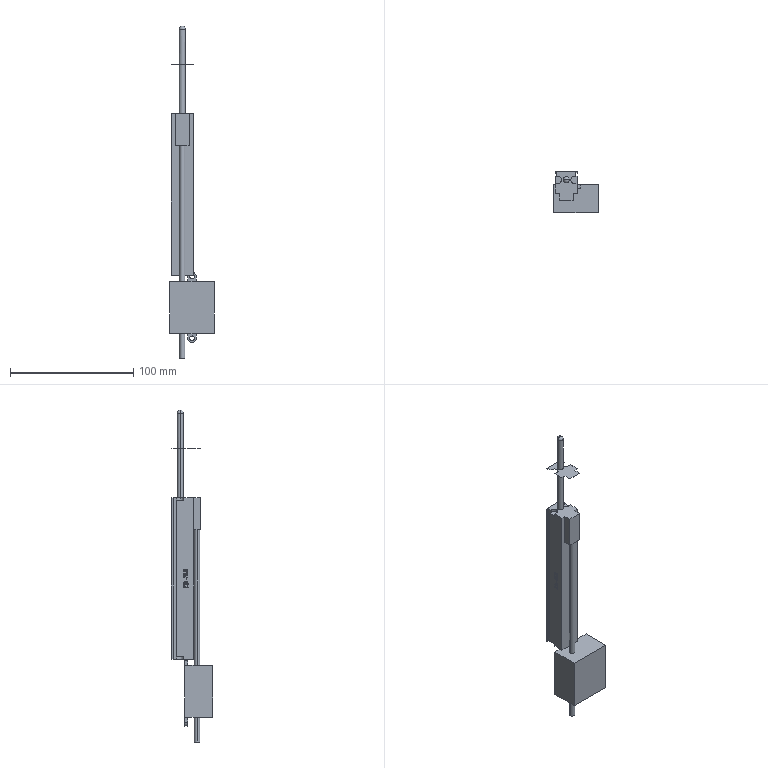Part | STEP file | KTC linear displacement sensor KTC2-50MM | 1 solid | 291 faces | box 36 x 33.3 x 269 mm | volume 80429 mm3 | plane 194 | spline 72 | cylinder 23 | sphere 2 | commonest cylinder face diameters 6 x9 4.5 x4 5 x4 3.7 x3 6.7 x3